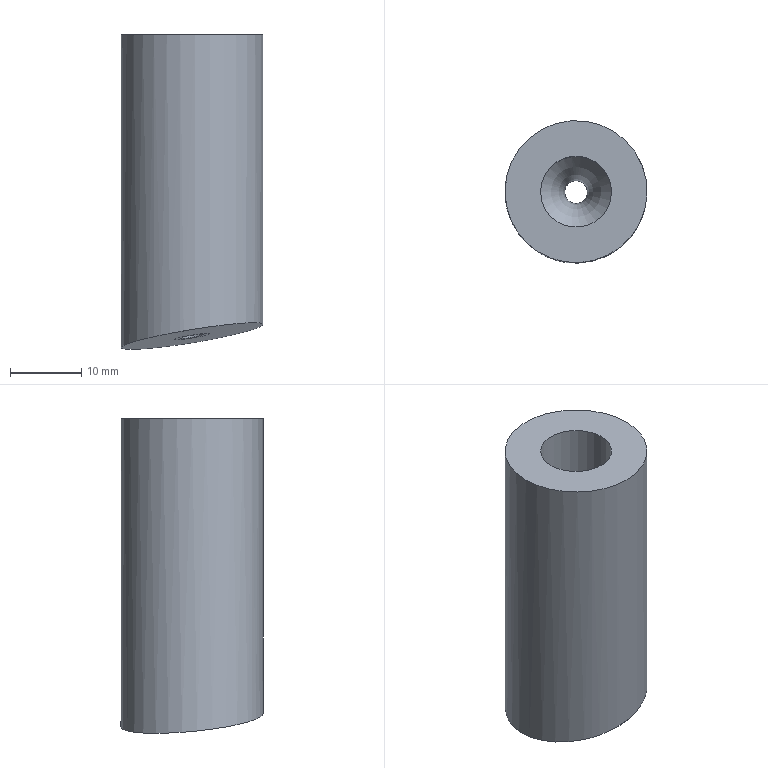Part | NX | features solid 2 | 1 solid | 9 faces | box 20 x 20 x 44.29 mm | volume 10691 mm3 | spline 4 | cylinder 3 | plane 1 | torus 1 | commonest cylinder face diameters 3.2 x1 10 x1 20 x1
STEP:
#1=CARTESIAN_POINT('',(334.711,-390.087,-19.));
#2=VERTEX_POINT('',#1);
#3=CARTESIAN_POINT('',(344.711,-390.087,-19.));
#4=DIRECTION('',(0.,0.,-1.));
#5=DIRECTION('',(-1.,0.,0.));
#6=AXIS2_PLACEMENT_3D('',#3,#4,#5);
#7=CIRCLE('',#6,10.);
#8=EDGE_CURVE('',#2,#2,#7,.T.);
#9=ORIENTED_EDGE('',*,*,#8,.F.);
#10=EDGE_LOOP('',(#9));
#11=FACE_BOUND('',#10,.T.);
#12=CARTESIAN_POINT('',(339.711,-390.087,-19.));
#13=VERTEX_POINT('',#12);
#14=CARTESIAN_POINT('',(344.711,-390.087,-19.));
#15=DIRECTION('',(0.,0.,-1.));
#16=DIRECTION('',(-1.,0.,0.));
#17=AXIS2_PLACEMENT_3D('',#14,#15,#16);
#18=CIRCLE('',#17,5.);
#19=EDGE_CURVE('',#13,#13,#18,.F.);
#20=ORIENTED_EDGE('',*,*,#19,.F.);
#21=EDGE_LOOP('',(#20));
#22=FACE_BOUND('',#21,.T.);
#23=CARTESIAN_POINT('',(344.711,-390.087,-19.));
#24=DIRECTION('',(0.,0.,-1.));
#25=DIRECTION('',(-1.,0.,0.));
#26=AXIS2_PLACEMENT_3D('',#23,#24,#25);
#27=PLANE('',#26);
#28=ADVANCED_FACE('',(#11,#22),#27,.F.);
#29=CARTESIAN_POINT('',(345.089,-400.08,-60.446));
#30=VERTEX_POINT('',#29);
#31=CARTESIAN_POINT('',(342.968,-399.934,-60.804));
#32=VERTEX_POINT('',#31);
#33=CARTESIAN_POINT('',(345.099,-400.08,-60.444));
#34=CARTESIAN_POINT('',(347.632,-399.982,-60.04));
#35=CARTESIAN_POINT('',(352.593,-397.791,-59.418));
#36=CARTESIAN_POINT('',(355.735,-390.139,-59.593));
#37=CARTESIAN_POINT('',(352.733,-382.585,-60.819));
#38=CARTESIAN_POINT('',(345.484,-379.126,-62.355));
#39=CARTESIAN_POINT('',(337.707,-381.575,-63.367));
#40=CARTESIAN_POINT('',(333.76,-388.826,-63.296));
#41=CARTESIAN_POINT('',(335.924,-396.696,-62.227));
#42=CARTESIAN_POINT('',(340.51,-399.5,-61.241));
#43=CARTESIAN_POINT('',(342.972,-399.935,-60.803));
#44=B_SPLINE_CURVE_WITH_KNOTS('',3,(#33,#34,#35,#36,#37,#38,#39,#40,#41,#42,#43),.UNSPECIFIED.,.F.,.F.,(4,1,1,1,1,1,1,1,4),(0.04777,0.05538,0.063,0.07061,0.07823,0.08584,0.09345,0.1011,0.1087),.UNSPECIFIED.);
#45=EDGE_CURVE('',#30,#32,#44,.T.);
#46=ORIENTED_EDGE('',*,*,#45,.T.);
#47=CARTESIAN_POINT('',(343.528,-400.017,-60.705));
#48=VERTEX_POINT('',#47);
#49=CARTESIAN_POINT('',(342.965,-399.933,-60.804));
#50=CARTESIAN_POINT('',(343.152,-399.967,-60.771));
#51=CARTESIAN_POINT('',(343.339,-399.994,-60.738));
#52=CARTESIAN_POINT('',(343.528,-400.017,-60.705));
#53=B_SPLINE_CURVE_WITH_KNOTS('',3,(#49,#50,#51,#52),.UNSPECIFIED.,.F.,.F.,(4,4),(0.,0.0005776),.UNSPECIFIED.);
#54=EDGE_CURVE('',#32,#48,#53,.T.);
#55=ORIENTED_EDGE('',*,*,#54,.T.);
#56=CARTESIAN_POINT('',(343.528,-400.017,-60.705));
#57=CARTESIAN_POINT('',(344.043,-400.078,-60.615));
#58=CARTESIAN_POINT('',(344.56,-400.1,-60.53));
#59=CARTESIAN_POINT('',(345.079,-400.08,-60.447));
#60=B_SPLINE_CURVE_WITH_KNOTS('',3,(#56,#57,#58,#59),.UNSPECIFIED.,.F.,.F.,(4,4),(0.,0.001574),.UNSPECIFIED.);
#61=EDGE_CURVE('',#48,#30,#60,.T.);
#62=ORIENTED_EDGE('',*,*,#61,.T.);
#63=EDGE_LOOP('',(#46,#55,#62));
#64=FACE_BOUND('',#63,.T.);
#65=ORIENTED_EDGE('',*,*,#8,.T.);
#66=EDGE_LOOP('',(#65));
#67=FACE_BOUND('',#66,.T.);
#68=CARTESIAN_POINT('',(344.711,-390.087,-69.));
#69=DIRECTION('',(0.,0.,1.));
#70=DIRECTION('',(1.,0.,0.));
#71=AXIS2_PLACEMENT_3D('',#68,#69,#70);
#72=CYLINDRICAL_SURFACE('',#71,10.);
#73=ADVANCED_FACE('',(#64,#67),#72,.T.);
#74=CARTESIAN_POINT('',(339.711,-390.087,-49.705));
#75=VERTEX_POINT('',#74);
#76=CARTESIAN_POINT('',(344.711,-390.087,-49.705));
#77=DIRECTION('',(0.,0.,-1.));
#78=DIRECTION('',(-1.,0.,0.));
#79=AXIS2_PLACEMENT_3D('',#76,#77,#78);
#80=CIRCLE('',#79,5.);
#81=EDGE_CURVE('',#75,#75,#80,.F.);
#82=ORIENTED_EDGE('',*,*,#81,.F.);
#83=EDGE_LOOP('',(#82));
#84=FACE_BOUND('',#83,.T.);
#85=ORIENTED_EDGE('',*,*,#19,.T.);
#86=EDGE_LOOP('',(#85));
#87=FACE_BOUND('',#86,.T.);
#88=CARTESIAN_POINT('',(344.711,-390.087,11.));
#89=DIRECTION('',(0.,0.,-1.));
#90=DIRECTION('',(0.,-1.,0.));
#91=AXIS2_PLACEMENT_3D('',#88,#89,#90);
#92=CYLINDRICAL_SURFACE('',#91,5.);
#93=ADVANCED_FACE('',(#84,#87),#92,.F.);
#94=CARTESIAN_POINT('',(344.711,-388.487,-61.607));
#95=VERTEX_POINT('',#94);
#96=CARTESIAN_POINT('',(343.453,-388.832,-61.779));
#97=CARTESIAN_POINT('',(344.716,-388.316,-61.623));
#98=CARTESIAN_POINT('',(345.954,-388.828,-61.372));
#99=CARTESIAN_POINT('',(346.486,-390.068,-61.169));
#100=CARTESIAN_POINT('',(345.97,-391.342,-61.134));
#101=CARTESIAN_POINT('',(344.708,-391.858,-61.292));
#102=CARTESIAN_POINT('',(343.471,-391.348,-61.54));
#103=CARTESIAN_POINT('',(342.936,-390.107,-61.743));
#104=CARTESIAN_POINT('',(343.453,-388.832,-61.779));
#105=CARTESIAN_POINT('',(344.716,-388.316,-61.623));
#106=CARTESIAN_POINT('',(345.954,-388.828,-61.372));
#107=B_SPLINE_CURVE_WITH_KNOTS('',3,(#96,#97,#98,#99,#100,#101,#102,#103,#104,#105,#106),.UNSPECIFIED.,.T.,.F.,(1,1,1,1,1,1,1,1,1,1,1,1,1,1,1),(-0.003783,-0.002522,-0.001261,0.,0.001261,0.002522,0.003783,0.005044,0.006306,0.007567,0.008828,0.01009,0.01135,0.01261,0.01387),.UNSPECIFIED.);
#108=EDGE_CURVE('',#95,#95,#107,.T.);
#109=ORIENTED_EDGE('',*,*,#108,.T.);
#110=EDGE_LOOP('',(#109));
#111=FACE_BOUND('',#110,.T.);
#112=CARTESIAN_POINT('',(346.311,-390.087,-57.614));
#113=VERTEX_POINT('',#112);
#114=CARTESIAN_POINT('',(344.711,-390.087,-57.614));
#115=DIRECTION('',(0.,0.,1.));
#116=DIRECTION('',(1.,0.,0.));
#117=AXIS2_PLACEMENT_3D('',#114,#115,#116);
#118=CIRCLE('',#117,1.6);
#119=EDGE_CURVE('',#113,#113,#118,.F.);
#120=ORIENTED_EDGE('',*,*,#119,.F.);
#121=EDGE_LOOP('',(#120));
#122=FACE_BOUND('',#121,.T.);
#123=CARTESIAN_POINT('',(344.711,-390.087,-79.));
#124=DIRECTION('',(0.,0.,1.));
#125=DIRECTION('',(0.,1.,0.));
#126=AXIS2_PLACEMENT_3D('',#123,#124,#125);
#127=CYLINDRICAL_SURFACE('',#126,1.6);
#128=ADVANCED_FACE('',(#111,#122),#127,.F.);
#129=ORIENTED_EDGE('',*,*,#119,.T.);
#130=EDGE_LOOP('',(#129));
#131=FACE_BOUND('',#130,.T.);
#132=ORIENTED_EDGE('',*,*,#81,.T.);
#133=EDGE_LOOP('',(#132));
#134=FACE_BOUND('',#133,.T.);
#135=CARTESIAN_POINT('',(344.711,-390.087,-57.614));
#136=DIRECTION('',(0.,0.,1.));
#137=DIRECTION('',(1.,0.,0.));
#138=AXIS2_PLACEMENT_3D('',#135,#136,#137);
#139=TOROIDAL_SURFACE('',#138,12.5,10.9);
#140=ADVANCED_FACE('',(#131,#134),#139,.T.);
#141=CARTESIAN_POINT('',(346.239,-392.003,-61.027));
#142=VERTEX_POINT('',#141);
#143=CARTESIAN_POINT('',(343.2,-388.126,-61.886));
#144=VERTEX_POINT('',#143);
#145=CARTESIAN_POINT('',(346.239,-392.003,-61.027));
#146=CARTESIAN_POINT('',(345.699,-392.437,-61.075));
#147=CARTESIAN_POINT('',(344.381,-392.792,-61.257));
#148=CARTESIAN_POINT('',(342.569,-391.803,-61.643));
#149=CARTESIAN_POINT('',(342.014,-389.784,-61.921));
#150=CARTESIAN_POINT('',(342.657,-388.561,-61.932));
#151=CARTESIAN_POINT('',(343.2,-388.126,-61.886));
#152=B_SPLINE_CURVE_WITH_KNOTS('',3,(#145,#146,#147,#148,#149,#150,#151),.UNSPECIFIED.,.F.,.F.,(4,1,1,1,4),(0.,0.25,0.5,0.75,1.),.UNSPECIFIED.);
#153=EDGE_CURVE('',#142,#144,#152,.T.);
#154=ORIENTED_EDGE('',*,*,#153,.F.);
#155=CARTESIAN_POINT('',(343.2,-388.126,-61.886));
#156=CARTESIAN_POINT('',(343.741,-387.692,-61.839));
#157=CARTESIAN_POINT('',(345.059,-387.337,-61.658));
#158=CARTESIAN_POINT('',(346.87,-388.326,-61.268));
#159=CARTESIAN_POINT('',(347.425,-390.344,-60.988));
#160=CARTESIAN_POINT('',(346.782,-391.568,-60.979));
#161=CARTESIAN_POINT('',(346.239,-392.003,-61.027));
#162=B_SPLINE_CURVE_WITH_KNOTS('',3,(#155,#156,#157,#158,#159,#160,#161),.UNSPECIFIED.,.F.,.F.,(4,1,1,1,4),(0.,0.25,0.5,0.75,1.),.UNSPECIFIED.);
#163=EDGE_CURVE('',#144,#142,#162,.T.);
#164=ORIENTED_EDGE('',*,*,#163,.F.);
#165=EDGE_LOOP('',(#154,#164));
#166=FACE_BOUND('',#165,.T.);
#167=CARTESIAN_POINT('',(343.53,-399.942,-60.712));
#168=VERTEX_POINT('',#167);
#169=CARTESIAN_POINT('',(342.968,-399.935,-60.804));
#170=CARTESIAN_POINT('',(343.156,-399.937,-60.773));
#171=CARTESIAN_POINT('',(343.343,-399.94,-60.743));
#172=CARTESIAN_POINT('',(343.53,-399.942,-60.712));
#173=B_SPLINE_CURVE_WITH_KNOTS('',3,(#169,#170,#171,#172),.UNSPECIFIED.,.F.,.F.,(4,4),(0.9646,1.),.UNSPECIFIED.);
#174=EDGE_CURVE('',#32,#168,#173,.T.);
#175=ORIENTED_EDGE('',*,*,#174,.F.);
#176=ORIENTED_EDGE('',*,*,#45,.F.);
#177=CARTESIAN_POINT('',(343.53,-399.942,-60.712));
#178=CARTESIAN_POINT('',(344.06,-399.95,-60.626));
#179=CARTESIAN_POINT('',(344.58,-399.996,-60.537));
#180=CARTESIAN_POINT('',(345.089,-400.078,-60.446));
#181=B_SPLINE_CURVE_WITH_KNOTS('',3,(#177,#178,#179,#180),.UNSPECIFIED.,.F.,.F.,(4,4),(0.,0.1415),.UNSPECIFIED.);
#182=EDGE_CURVE('',#168,#30,#181,.T.);
#183=ORIENTED_EDGE('',*,*,#182,.F.);
#184=EDGE_LOOP('',(#175,#176,#183));
#185=FACE_BOUND('',#184,.T.);
#186=CARTESIAN_POINT('',(354.757,-399.816,-58.843));
#187=CARTESIAN_POINT('',(350.702,-399.98,-59.532));
#188=CARTESIAN_POINT('',(346.643,-400.141,-60.199));
#189=CARTESIAN_POINT('',(342.58,-400.301,-60.844));
#190=CARTESIAN_POINT('',(338.514,-400.458,-61.468));
#191=CARTESIAN_POINT('',(334.444,-400.612,-62.072));
#192=CARTESIAN_POINT('',(354.791,-395.757,-59.227));
#193=CARTESIAN_POINT('',(350.736,-395.919,-59.917));
#194=CARTESIAN_POINT('',(346.677,-396.078,-60.585));
#195=CARTESIAN_POINT('',(342.614,-396.236,-61.23));
#196=CARTESIAN_POINT('',(338.548,-396.391,-61.855));
#197=CARTESIAN_POINT('',(334.479,-396.544,-62.459));
#198=CARTESIAN_POINT('',(354.824,-391.696,-59.607));
#199=CARTESIAN_POINT('',(350.769,-391.857,-60.297));
#200=CARTESIAN_POINT('',(346.711,-392.015,-60.965));
#201=CARTESIAN_POINT('',(342.648,-392.17,-61.612));
#202=CARTESIAN_POINT('',(338.582,-392.324,-62.237));
#203=CARTESIAN_POINT('',(334.513,-392.475,-62.841));
#204=CARTESIAN_POINT('',(354.857,-387.636,-59.981));
#205=CARTESIAN_POINT('',(350.803,-387.794,-60.672));
#206=CARTESIAN_POINT('',(346.744,-387.951,-61.341));
#207=CARTESIAN_POINT('',(342.682,-388.105,-61.987));
#208=CARTESIAN_POINT('',(338.616,-388.256,-62.613));
#209=CARTESIAN_POINT('',(334.547,-388.406,-63.217));
#210=CARTESIAN_POINT('',(354.89,-383.575,-60.35));
#211=CARTESIAN_POINT('',(350.835,-383.731,-61.042));
#212=CARTESIAN_POINT('',(346.777,-383.886,-61.711));
#213=CARTESIAN_POINT('',(342.715,-384.038,-62.358));
#214=CARTESIAN_POINT('',(338.649,-384.188,-62.984));
#215=CARTESIAN_POINT('',(334.58,-384.336,-63.588));
#216=CARTESIAN_POINT('',(354.922,-379.513,-60.714));
#217=CARTESIAN_POINT('',(350.868,-379.668,-61.406));
#218=CARTESIAN_POINT('',(346.81,-379.82,-62.076));
#219=CARTESIAN_POINT('',(342.748,-379.971,-62.723));
#220=CARTESIAN_POINT('',(338.682,-380.119,-63.349));
#221=CARTESIAN_POINT('',(334.613,-380.265,-63.954));
#222=B_SPLINE_SURFACE_WITH_KNOTS('',5,5,((#186,#187,#188,#189,#190,#191),(#192,#193,#194,#195,#196,#197),(#198,#199,#200,#201,#202,#203),(#204,#205,#206,#207,#208,#209),(#210,#211,#212,#213,#214,#215),(#216,#217,#218,#219,#220,#221)),.UNSPECIFIED.,.F.,.F.,.F.,(6,6),(6,6),(0.245,0.9845),(0.6605,0.9139),.PIECEWISE_BEZIER_KNOTS.);
#223=ADVANCED_FACE('',(#166,#185),#222,.F.);
#224=ORIENTED_EDGE('',*,*,#61,.F.);
#225=CARTESIAN_POINT('',(343.53,-399.942,-60.712));
#226=CARTESIAN_POINT('',(343.529,-399.967,-60.71));
#227=CARTESIAN_POINT('',(343.529,-399.992,-60.708));
#228=CARTESIAN_POINT('',(343.528,-400.017,-60.705));
#229=B_SPLINE_CURVE_WITH_KNOTS('',3,(#225,#226,#227,#228),.UNSPECIFIED.,.F.,.F.,(4,4),(0.,0.008385),.UNSPECIFIED.);
#230=EDGE_CURVE('',#168,#48,#229,.T.);
#231=ORIENTED_EDGE('',*,*,#230,.F.);
#232=ORIENTED_EDGE('',*,*,#182,.T.);
#233=EDGE_LOOP('',(#224,#231,#232));
#234=FACE_BOUND('',#233,.T.);
#235=CARTESIAN_POINT('',(345.098,-400.083,-60.444));
#236=CARTESIAN_POINT('',(345.094,-400.105,-60.443));
#237=CARTESIAN_POINT('',(345.09,-400.127,-60.441));
#238=CARTESIAN_POINT('',(345.086,-400.148,-60.439));
#239=CARTESIAN_POINT('',(345.082,-400.17,-60.438));
#240=CARTESIAN_POINT('',(345.078,-400.192,-60.436));
#241=CARTESIAN_POINT('',(344.788,-400.032,-60.5));
#242=CARTESIAN_POINT('',(344.785,-400.054,-60.498));
#243=CARTESIAN_POINT('',(344.782,-400.075,-60.496));
#244=CARTESIAN_POINT('',(344.778,-400.097,-60.495));
#245=CARTESIAN_POINT('',(344.775,-400.119,-60.493));
#246=CARTESIAN_POINT('',(344.772,-400.141,-60.491));
#247=CARTESIAN_POINT('',(344.476,-399.992,-60.554));
#248=CARTESIAN_POINT('',(344.473,-400.014,-60.553));
#249=CARTESIAN_POINT('',(344.471,-400.036,-60.551));
#250=CARTESIAN_POINT('',(344.468,-400.057,-60.549));
#251=CARTESIAN_POINT('',(344.465,-400.079,-60.547));
#252=CARTESIAN_POINT('',(344.463,-400.101,-60.545));
#253=CARTESIAN_POINT('',(344.162,-399.964,-60.608));
#254=CARTESIAN_POINT('',(344.16,-399.985,-60.606));
#255=CARTESIAN_POINT('',(344.158,-400.007,-60.604));
#256=CARTESIAN_POINT('',(344.156,-400.029,-60.602));
#257=CARTESIAN_POINT('',(344.154,-400.051,-60.6));
#258=CARTESIAN_POINT('',(344.152,-400.073,-60.598));
#259=CARTESIAN_POINT('',(343.846,-399.947,-60.661));
#260=CARTESIAN_POINT('',(343.845,-399.969,-60.659));
#261=CARTESIAN_POINT('',(343.844,-399.991,-60.657));
#262=CARTESIAN_POINT('',(343.842,-400.012,-60.655));
#263=CARTESIAN_POINT('',(343.841,-400.034,-60.653));
#264=CARTESIAN_POINT('',(343.84,-400.056,-60.65));
#265=CARTESIAN_POINT('',(343.53,-399.942,-60.712));
#266=CARTESIAN_POINT('',(343.529,-399.964,-60.71));
#267=CARTESIAN_POINT('',(343.529,-399.986,-60.708));
#268=CARTESIAN_POINT('',(343.528,-400.008,-60.706));
#269=CARTESIAN_POINT('',(343.527,-400.029,-60.704));
#270=CARTESIAN_POINT('',(343.527,-400.051,-60.701));
#271=B_SPLINE_SURFACE_WITH_KNOTS('',5,5,((#235,#236,#237,#238,#239,#240),(#241,#242,#243,#244,#245,#246),(#247,#248,#249,#250,#251,#252),(#253,#254,#255,#256,#257,#258),(#259,#260,#261,#262,#263,#264),(#265,#266,#267,#268,#269,#270)),.UNSPECIFIED.,.F.,.F.,.F.,(6,6),(6,6),(0.8654,1.),(0.,0.01224),.PIECEWISE_BEZIER_KNOTS.);
#272=ADVANCED_FACE('',(#234),#271,.F.);
#273=ORIENTED_EDGE('',*,*,#54,.F.);
#274=ORIENTED_EDGE('',*,*,#174,.T.);
#275=ORIENTED_EDGE('',*,*,#230,.T.);
#276=EDGE_LOOP('',(#273,#274,#275));
#277=FACE_BOUND('',#276,.T.);
#278=CARTESIAN_POINT('',(342.962,-399.933,-60.805));
#279=CARTESIAN_POINT('',(342.961,-399.948,-60.803));
#280=CARTESIAN_POINT('',(342.961,-399.964,-60.802));
#281=CARTESIAN_POINT('',(342.96,-399.979,-60.801));
#282=CARTESIAN_POINT('',(342.96,-399.994,-60.799));
#283=CARTESIAN_POINT('',(342.959,-400.009,-60.798));
#284=CARTESIAN_POINT('',(343.075,-399.935,-60.786));
#285=CARTESIAN_POINT('',(343.075,-399.95,-60.785));
#286=CARTESIAN_POINT('',(343.074,-399.965,-60.784));
#287=CARTESIAN_POINT('',(343.074,-399.98,-60.782));
#288=CARTESIAN_POINT('',(343.073,-399.995,-60.781));
#289=CARTESIAN_POINT('',(343.073,-400.01,-60.779));
#290=CARTESIAN_POINT('',(343.189,-399.937,-60.768));
#291=CARTESIAN_POINT('',(343.189,-399.952,-60.767));
#292=CARTESIAN_POINT('',(343.188,-399.967,-60.765));
#293=CARTESIAN_POINT('',(343.188,-399.982,-60.764));
#294=CARTESIAN_POINT('',(343.187,-399.997,-60.762));
#295=CARTESIAN_POINT('',(343.187,-400.012,-60.761));
#296=CARTESIAN_POINT('',(343.303,-399.939,-60.749));
#297=CARTESIAN_POINT('',(343.302,-399.954,-60.748));
#298=CARTESIAN_POINT('',(343.302,-399.969,-60.747));
#299=CARTESIAN_POINT('',(343.301,-399.984,-60.745));
#300=CARTESIAN_POINT('',(343.301,-399.999,-60.744));
#301=CARTESIAN_POINT('',(343.3,-400.014,-60.742));
#302=CARTESIAN_POINT('',(343.416,-399.94,-60.731));
#303=CARTESIAN_POINT('',(343.416,-399.955,-60.73));
#304=CARTESIAN_POINT('',(343.416,-399.97,-60.728));
#305=CARTESIAN_POINT('',(343.415,-399.986,-60.727));
#306=CARTESIAN_POINT('',(343.415,-400.001,-60.725));
#307=CARTESIAN_POINT('',(343.414,-400.016,-60.724));
#308=CARTESIAN_POINT('',(343.53,-399.942,-60.712));
#309=CARTESIAN_POINT('',(343.53,-399.957,-60.711));
#310=CARTESIAN_POINT('',(343.529,-399.972,-60.71));
#311=CARTESIAN_POINT('',(343.529,-399.987,-60.708));
#312=CARTESIAN_POINT('',(343.528,-400.002,-60.707));
#313=CARTESIAN_POINT('',(343.528,-400.017,-60.705));
#314=B_SPLINE_SURFACE_WITH_KNOTS('',5,5,((#278,#279,#280,#281,#282,#283),(#284,#285,#286,#287,#288,#289),(#290,#291,#292,#293,#294,#295),(#296,#297,#298,#299,#300,#301),(#302,#303,#304,#305,#306,#307),(#308,#309,#310,#311,#312,#313)),.UNSPECIFIED.,.F.,.F.,.F.,(6,6),(6,6),(0.9641,1.),(0.,0.008435),.PIECEWISE_BEZIER_KNOTS.);
#315=ADVANCED_FACE('',(#277),#314,.T.);
#316=ORIENTED_EDGE('',*,*,#153,.T.);
#317=ORIENTED_EDGE('',*,*,#163,.T.);
#318=EDGE_LOOP('',(#316,#317));
#319=FACE_BOUND('',#318,.T.);
#320=ORIENTED_EDGE('',*,*,#108,.F.);
#321=EDGE_LOOP('',(#320));
#322=FACE_BOUND('',#321,.T.);
#323=CARTESIAN_POINT('',(347.237,-392.615,-60.805));
#324=CARTESIAN_POINT('',(346.211,-392.655,-60.971));
#325=CARTESIAN_POINT('',(345.184,-392.694,-61.136));
#326=CARTESIAN_POINT('',(344.158,-392.734,-61.299));
#327=CARTESIAN_POINT('',(343.131,-392.773,-61.461));
#328=CARTESIAN_POINT('',(342.103,-392.812,-61.622));
#329=CARTESIAN_POINT('',(347.246,-391.571,-60.902));
#330=CARTESIAN_POINT('',(346.219,-391.611,-61.068));
#331=CARTESIAN_POINT('',(345.193,-391.651,-61.233));
#332=CARTESIAN_POINT('',(344.166,-391.69,-61.396));
#333=CARTESIAN_POINT('',(343.139,-391.729,-61.558));
#334=CARTESIAN_POINT('',(342.112,-391.768,-61.719));
#335=CARTESIAN_POINT('',(347.254,-390.528,-60.999));
#336=CARTESIAN_POINT('',(346.228,-390.567,-61.165));
#337=CARTESIAN_POINT('',(345.202,-390.607,-61.33));
#338=CARTESIAN_POINT('',(344.175,-390.646,-61.493));
#339=CARTESIAN_POINT('',(343.148,-390.685,-61.655));
#340=CARTESIAN_POINT('',(342.121,-390.724,-61.816));
#341=CARTESIAN_POINT('',(347.263,-389.484,-61.095));
#342=CARTESIAN_POINT('',(346.237,-389.524,-61.261));
#343=CARTESIAN_POINT('',(345.21,-389.563,-61.426));
#344=CARTESIAN_POINT('',(344.183,-389.602,-61.59));
#345=CARTESIAN_POINT('',(343.156,-389.641,-61.752));
#346=CARTESIAN_POINT('',(342.129,-389.68,-61.912));
#347=CARTESIAN_POINT('',(347.271,-388.441,-61.191));
#348=CARTESIAN_POINT('',(346.245,-388.48,-61.357));
#349=CARTESIAN_POINT('',(345.219,-388.519,-61.522));
#350=CARTESIAN_POINT('',(344.192,-388.558,-61.686));
#351=CARTESIAN_POINT('',(343.165,-388.597,-61.848));
#352=CARTESIAN_POINT('',(342.138,-388.635,-62.009));
#353=CARTESIAN_POINT('',(347.28,-387.397,-61.287));
#354=CARTESIAN_POINT('',(346.254,-387.436,-61.453));
#355=CARTESIAN_POINT('',(345.227,-387.475,-61.618));
#356=CARTESIAN_POINT('',(344.201,-387.514,-61.782));
#357=CARTESIAN_POINT('',(343.174,-387.553,-61.944));
#358=CARTESIAN_POINT('',(342.146,-387.591,-62.104));
#359=B_SPLINE_SURFACE_WITH_KNOTS('',5,5,((#323,#324,#325,#326,#327,#328),(#329,#330,#331,#332,#333,#334),(#335,#336,#337,#338,#339,#340),(#341,#342,#343,#344,#345,#346),(#347,#348,#349,#350,#351,#352),(#353,#354,#355,#356,#357,#358)),.UNSPECIFIED.,.F.,.F.,.F.,(6,6),(6,6),(0.5181,0.7081),(0.7552,0.8193),.PIECEWISE_BEZIER_KNOTS.);
#360=ADVANCED_FACE('',(#319,#322),#359,.F.);
#361=CLOSED_SHELL('',(#28,#73,#93,#128,#140,#223,#272,#315,#360));
#362=MANIFOLD_SOLID_BREP('',#361);
#363=(LENGTH_UNIT()NAMED_UNIT(*)SI_UNIT(.MILLI.,.METRE.));
#364=UNCERTAINTY_MEASURE_WITH_UNIT(LENGTH_MEASURE(0.07365),#363,'','');
#365=(NAMED_UNIT(*)PLANE_ANGLE_UNIT()SI_UNIT($,.RADIAN.));
#366=(NAMED_UNIT(*)SI_UNIT($,.STERADIAN.)SOLID_ANGLE_UNIT());
#367=(GEOMETRIC_REPRESENTATION_CONTEXT(3)GLOBAL_UNCERTAINTY_ASSIGNED_CONTEXT((#364))GLOBAL_UNIT_ASSIGNED_CONTEXT((#363,#365,#366))REPRESENTATION_CONTEXT('',''));
#368=ADVANCED_BREP_SHAPE_REPRESENTATION('',(#362),#367);